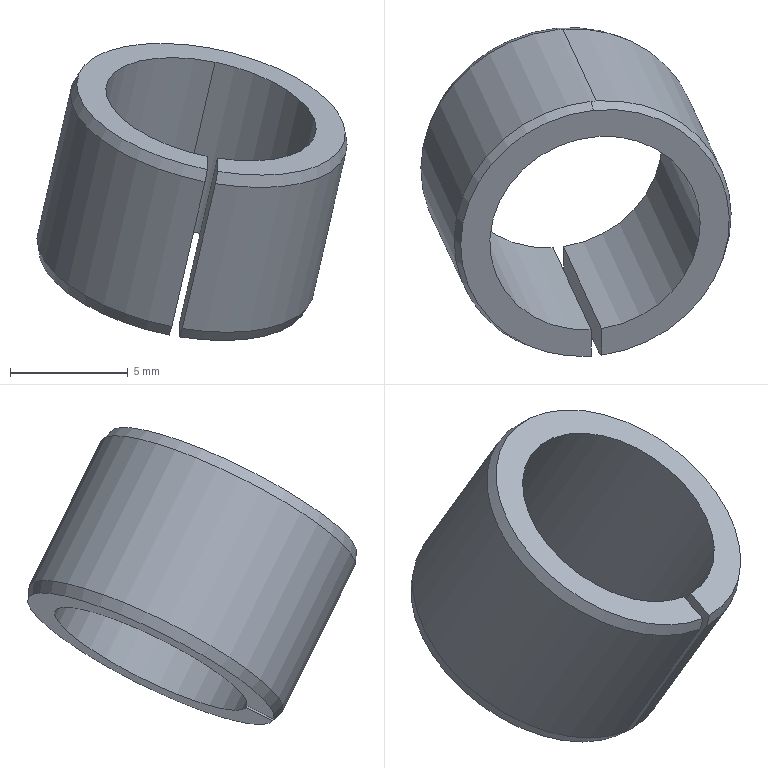Part | SolidWorks | features BaseBody 1 | 1 solid | 12 faces | box 13.154 x 13.951 x 12.601 mm | volume 373.279 mm3 | cone 4 | cylinder 4 | plane 4 | commonest cylinder face diameters 9.11 x2 11.99 x2
STEP:
#1=CARTESIAN_POINT('',(1949.772,-211.955,916.36));
#2=VERTEX_POINT('',#1);
#3=CARTESIAN_POINT('',(1949.419,-201.584,921.597));
#4=VERTEX_POINT('',#3);
#5=CARTESIAN_POINT('',(1949.485,-206.783,918.997));
#6=DIRECTION('',(0.2015,-0.436,0.8771));
#7=DIRECTION('',(0.9794,0.1001,-0.1752));
#8=AXIS2_PLACEMENT_3D('',#5,#6,#7);
#9=CIRCLE('',#8,5.813);
#10=EDGE_CURVE('',#2,#4,#9,.T.);
#11=ORIENTED_EDGE('',*,*,#10,.T.);
#12=CARTESIAN_POINT('',(1949.518,-201.639,922.117));
#13=VERTEX_POINT('',#12);
#14=CARTESIAN_POINT('',(1946.268,-199.819,904.989));
#15=DIRECTION('',(0.1854,-0.1038,0.9772));
#16=VECTOR('',#15,1000.);
#17=LINE('',#14,#16);
#18=EDGE_CURVE('',#4,#13,#17,.T.);
#19=ORIENTED_EDGE('',*,*,#18,.T.);
#20=CARTESIAN_POINT('',(1949.738,-201.62,922.076));
#21=VERTEX_POINT('',#20);
#22=CARTESIAN_POINT('',(1949.586,-207.001,919.436));
#23=DIRECTION('',(0.2015,-0.436,0.8771));
#24=DIRECTION('',(0.9794,0.1001,-0.1752));
#25=AXIS2_PLACEMENT_3D('',#22,#23,#24);
#26=CIRCLE('',#25,5.995);
#27=EDGE_CURVE('',#21,#13,#26,.T.);
#28=ORIENTED_EDGE('',*,*,#27,.F.);
#29=CARTESIAN_POINT('',(1949.875,-212.336,916.717));
#30=VERTEX_POINT('',#29);
#31=CARTESIAN_POINT('',(1949.586,-207.001,919.436));
#32=DIRECTION('',(0.2015,-0.436,0.8771));
#33=DIRECTION('',(0.9794,0.1001,-0.1752));
#34=AXIS2_PLACEMENT_3D('',#31,#32,#33);
#35=CIRCLE('',#34,5.995);
#36=EDGE_CURVE('',#30,#21,#35,.T.);
#37=ORIENTED_EDGE('',*,*,#36,.F.);
#38=CARTESIAN_POINT('',(1949.824,-212.146,916.539));
#39=DIRECTION('',(-0.1932,0.7158,-0.6711));
#40=VECTOR('',#39,1000.);
#41=LINE('',#38,#40);
#42=EDGE_CURVE('',#30,#2,#41,.T.);
#43=ORIENTED_EDGE('',*,*,#42,.T.);
#44=EDGE_LOOP('',(#11,#19,#28,#37,#43));
#45=FACE_OUTER_BOUND('',#44,.T.);
#46=CARTESIAN_POINT('',(2147.735,-635.836,1782.087));
#47=DIRECTION('',(0.2015,-0.436,0.8771));
#48=DIRECTION('',(-0.01144,0.8943,0.4472));
#49=AXIS2_PLACEMENT_3D('',#46,#47,#48);
#50=CONICAL_SURFACE('',#49,363.97,0.3491);
#51=ADVANCED_FACE('',(#45),#50,.T.);
#52=ORIENTED_EDGE('',*,*,#36,.T.);
#53=CARTESIAN_POINT('',(1951.148,-204.672,928.215));
#54=VERTEX_POINT('',#53);
#55=CARTESIAN_POINT('',(1950.443,-203.146,925.145));
#56=DIRECTION('',(0.2015,-0.436,0.8771));
#57=VECTOR('',#56,1000.);
#58=LINE('',#55,#57);
#59=EDGE_CURVE('',#21,#54,#58,.T.);
#60=ORIENTED_EDGE('',*,*,#59,.T.);
#61=CARTESIAN_POINT('',(1951.285,-215.388,922.857));
#62=VERTEX_POINT('',#61);
#63=CARTESIAN_POINT('',(1950.996,-210.053,925.576));
#64=DIRECTION('',(0.2015,-0.436,0.8771));
#65=DIRECTION('',(0.9794,0.1001,-0.1752));
#66=AXIS2_PLACEMENT_3D('',#63,#64,#65);
#67=CIRCLE('',#66,5.995);
#68=EDGE_CURVE('',#62,#54,#67,.T.);
#69=ORIENTED_EDGE('',*,*,#68,.F.);
#70=CARTESIAN_POINT('',(1950.58,-213.862,919.787));
#71=DIRECTION('',(-0.2015,0.436,-0.8771));
#72=VECTOR('',#71,1000.);
#73=LINE('',#70,#72);
#74=EDGE_CURVE('',#62,#30,#73,.T.);
#75=ORIENTED_EDGE('',*,*,#74,.T.);
#76=EDGE_LOOP('',(#52,#60,#69,#75));
#77=FACE_OUTER_BOUND('',#76,.T.);
#78=CARTESIAN_POINT('',(1950.291,-208.527,922.506));
#79=DIRECTION('',(0.2015,-0.436,0.8771));
#80=DIRECTION('',(0.02532,0.8975,0.4403));
#81=AXIS2_PLACEMENT_3D('',#78,#79,#80);
#82=CYLINDRICAL_SURFACE('',#81,5.995);
#83=ADVANCED_FACE('',(#77),#82,.T.);
#84=CARTESIAN_POINT('',(1951.031,-205.072,928.614));
#85=VERTEX_POINT('',#84);
#86=CARTESIAN_POINT('',(1950.943,-215.488,923.456));
#87=VERTEX_POINT('',#86);
#88=CARTESIAN_POINT('',(1951.097,-210.271,926.014));
#89=DIRECTION('',(0.2015,-0.436,0.8771));
#90=DIRECTION('',(0.9794,0.1001,-0.1752));
#91=AXIS2_PLACEMENT_3D('',#88,#89,#90);
#92=CIRCLE('',#91,5.813);
#93=EDGE_CURVE('',#85,#87,#92,.T.);
#94=ORIENTED_EDGE('',*,*,#93,.F.);
#95=CARTESIAN_POINT('',(1950.928,-204.691,928.257));
#96=VERTEX_POINT('',#95);
#97=CARTESIAN_POINT('',(1954.315,-217.234,940.022));
#98=DIRECTION('',(-0.1932,0.7156,-0.6712));
#99=VECTOR('',#98,1000.);
#100=LINE('',#97,#99);
#101=EDGE_CURVE('',#85,#96,#100,.T.);
#102=ORIENTED_EDGE('',*,*,#101,.T.);
#103=CARTESIAN_POINT('',(1950.845,-215.433,922.936));
#104=VERTEX_POINT('',#103);
#105=CARTESIAN_POINT('',(1950.996,-210.053,925.576));
#106=DIRECTION('',(0.2015,-0.436,0.8771));
#107=DIRECTION('',(0.9794,0.1001,-0.1752));
#108=AXIS2_PLACEMENT_3D('',#105,#106,#107);
#109=CIRCLE('',#108,5.995);
#110=EDGE_CURVE('',#96,#104,#109,.T.);
#111=ORIENTED_EDGE('',*,*,#110,.T.);
#112=CARTESIAN_POINT('',(1950.894,-215.461,923.196));
#113=DIRECTION('',(0.1854,-0.1036,0.9772));
#114=VECTOR('',#113,1000.);
#115=LINE('',#112,#114);
#116=EDGE_CURVE('',#104,#87,#115,.T.);
#117=ORIENTED_EDGE('',*,*,#116,.T.);
#118=EDGE_LOOP('',(#94,#102,#111,#117));
#119=FACE_OUTER_BOUND('',#118,.T.);
#120=CARTESIAN_POINT('',(1752.847,218.782,62.925));
#121=DIRECTION('',(-0.2015,0.436,-0.8771));
#122=DIRECTION('',(-0.01144,0.8943,0.4472));
#123=AXIS2_PLACEMENT_3D('',#120,#121,#122);
#124=CONICAL_SURFACE('',#123,363.97,0.3491);
#125=ADVANCED_FACE('',(#119),#124,.T.);
#126=CARTESIAN_POINT('',(1949.317,-210.874,917.002));
#127=VERTEX_POINT('',#126);
#128=CARTESIAN_POINT('',(1949.654,-202.691,920.993));
#129=VERTEX_POINT('',#128);
#130=CARTESIAN_POINT('',(1949.485,-206.783,918.997));
#131=DIRECTION('',(-0.2015,0.436,-0.8771));
#132=DIRECTION('',(0.9794,0.1001,-0.1752));
#133=AXIS2_PLACEMENT_3D('',#130,#131,#132);
#134=CIRCLE('',#133,4.555);
#135=EDGE_CURVE('',#127,#129,#134,.T.);
#136=ORIENTED_EDGE('',*,*,#135,.T.);
#137=CARTESIAN_POINT('',(1951.266,-206.179,928.009));
#138=VERTEX_POINT('',#137);
#139=CARTESIAN_POINT('',(1950.46,-204.435,924.501));
#140=DIRECTION('',(0.2015,-0.436,0.8771));
#141=VECTOR('',#140,1000.);
#142=LINE('',#139,#141);
#143=EDGE_CURVE('',#129,#138,#142,.T.);
#144=ORIENTED_EDGE('',*,*,#143,.T.);
#145=CARTESIAN_POINT('',(1950.929,-214.362,924.019));
#146=VERTEX_POINT('',#145);
#147=CARTESIAN_POINT('',(1951.097,-210.271,926.014));
#148=DIRECTION('',(-0.2015,0.436,-0.8771));
#149=DIRECTION('',(0.9794,0.1001,-0.1752));
#150=AXIS2_PLACEMENT_3D('',#147,#148,#149);
#151=CIRCLE('',#150,4.555);
#152=EDGE_CURVE('',#146,#138,#151,.T.);
#153=ORIENTED_EDGE('',*,*,#152,.F.);
#154=CARTESIAN_POINT('',(1950.123,-212.618,920.511));
#155=DIRECTION('',(-0.2015,0.436,-0.8771));
#156=VECTOR('',#155,1000.);
#157=LINE('',#154,#156);
#158=EDGE_CURVE('',#146,#127,#157,.T.);
#159=ORIENTED_EDGE('',*,*,#158,.T.);
#160=EDGE_LOOP('',(#136,#144,#153,#159));
#161=FACE_OUTER_BOUND('',#160,.T.);
#162=CARTESIAN_POINT('',(1950.291,-208.527,922.506));
#163=DIRECTION('',(0.2015,-0.436,0.8771));
#164=DIRECTION('',(0.03695,0.8982,0.438));
#165=AXIS2_PLACEMENT_3D('',#162,#163,#164);
#166=CYLINDRICAL_SURFACE('',#165,4.555);
#167=ADVANCED_FACE('',(#161),#166,.F.);
#168=ORIENTED_EDGE('',*,*,#143,.F.);
#169=CARTESIAN_POINT('',(1949.758,-210.829,916.923));
#170=VERTEX_POINT('',#169);
#171=CARTESIAN_POINT('',(1949.485,-206.783,918.997));
#172=DIRECTION('',(-0.2015,0.436,-0.8771));
#173=DIRECTION('',(0.9794,0.1001,-0.1752));
#174=AXIS2_PLACEMENT_3D('',#171,#172,#173);
#175=CIRCLE('',#174,4.555);
#176=EDGE_CURVE('',#129,#170,#175,.T.);
#177=ORIENTED_EDGE('',*,*,#176,.T.);
#178=CARTESIAN_POINT('',(1951.37,-214.317,923.94));
#179=VERTEX_POINT('',#178);
#180=CARTESIAN_POINT('',(1950.564,-212.573,920.432));
#181=DIRECTION('',(-0.2015,0.436,-0.8771));
#182=VECTOR('',#181,1000.);
#183=LINE('',#180,#182);
#184=EDGE_CURVE('',#179,#170,#183,.T.);
#185=ORIENTED_EDGE('',*,*,#184,.F.);
#186=CARTESIAN_POINT('',(1951.097,-210.271,926.014));
#187=DIRECTION('',(-0.2015,0.436,-0.8771));
#188=DIRECTION('',(0.9794,0.1001,-0.1752));
#189=AXIS2_PLACEMENT_3D('',#186,#187,#188);
#190=CIRCLE('',#189,4.555);
#191=EDGE_CURVE('',#138,#179,#190,.T.);
#192=ORIENTED_EDGE('',*,*,#191,.F.);
#193=EDGE_LOOP('',(#168,#177,#185,#192));
#194=FACE_OUTER_BOUND('',#193,.T.);
#195=CARTESIAN_POINT('',(1950.291,-208.527,922.506));
#196=DIRECTION('',(0.2015,-0.436,0.8771));
#197=DIRECTION('',(0.03695,0.8982,0.438));
#198=AXIS2_PLACEMENT_3D('',#195,#196,#197);
#199=CYLINDRICAL_SURFACE('',#198,4.555);
#200=ADVANCED_FACE('',(#194),#199,.F.);
#201=CARTESIAN_POINT('',(1951.384,-215.443,923.377));
#202=VERTEX_POINT('',#201);
#203=CARTESIAN_POINT('',(1951.377,-214.88,923.659));
#204=DIRECTION('',(0.01144,-0.8943,-0.4472));
#205=VECTOR('',#204,1000.);
#206=LINE('',#203,#205);
#207=EDGE_CURVE('',#179,#202,#206,.T.);
#208=ORIENTED_EDGE('',*,*,#207,.T.);
#209=CARTESIAN_POINT('',(1951.097,-210.271,926.014));
#210=DIRECTION('',(0.2015,-0.436,0.8771));
#211=DIRECTION('',(0.9794,0.1001,-0.1752));
#212=AXIS2_PLACEMENT_3D('',#209,#210,#211);
#213=CIRCLE('',#212,5.813);
#214=EDGE_CURVE('',#202,#85,#213,.T.);
#215=ORIENTED_EDGE('',*,*,#214,.T.);
#216=ORIENTED_EDGE('',*,*,#93,.T.);
#217=CARTESIAN_POINT('',(1950.936,-214.925,923.737));
#218=DIRECTION('',(-0.01144,0.8943,0.4472));
#219=VECTOR('',#218,1000.);
#220=LINE('',#217,#219);
#221=EDGE_CURVE('',#87,#146,#220,.T.);
#222=ORIENTED_EDGE('',*,*,#221,.T.);
#223=ORIENTED_EDGE('',*,*,#152,.T.);
#224=ORIENTED_EDGE('',*,*,#191,.T.);
#225=EDGE_LOOP('',(#208,#215,#216,#222,#223,#224));
#226=FACE_OUTER_BOUND('',#225,.T.);
#227=CARTESIAN_POINT('',(1951.097,-210.271,926.014));
#228=DIRECTION('',(0.2015,-0.436,0.8771));
#229=DIRECTION('',(-0.9794,-0.1001,0.1752));
#230=AXIS2_PLACEMENT_3D('',#227,#228,#229);
#231=PLANE('',#230);
#232=ADVANCED_FACE('',(#226),#231,.T.);
#233=ORIENTED_EDGE('',*,*,#101,.F.);
#234=ORIENTED_EDGE('',*,*,#214,.F.);
#235=CARTESIAN_POINT('',(1951.335,-215.416,923.117));
#236=DIRECTION('',(-0.1854,0.1036,-0.9772));
#237=VECTOR('',#236,1000.);
#238=LINE('',#235,#237);
#239=EDGE_CURVE('',#202,#62,#238,.T.);
#240=ORIENTED_EDGE('',*,*,#239,.T.);
#241=ORIENTED_EDGE('',*,*,#68,.T.);
#242=CARTESIAN_POINT('',(1950.996,-210.053,925.576));
#243=DIRECTION('',(0.2015,-0.436,0.8771));
#244=DIRECTION('',(0.9794,0.1001,-0.1752));
#245=AXIS2_PLACEMENT_3D('',#242,#243,#244);
#246=CIRCLE('',#245,5.995);
#247=EDGE_CURVE('',#54,#96,#246,.T.);
#248=ORIENTED_EDGE('',*,*,#247,.T.);
#249=EDGE_LOOP('',(#233,#234,#240,#241,#248));
#250=FACE_OUTER_BOUND('',#249,.T.);
#251=CARTESIAN_POINT('',(1752.847,218.782,62.925));
#252=DIRECTION('',(-0.2015,0.436,-0.8771));
#253=DIRECTION('',(-0.01144,0.8943,0.4472));
#254=AXIS2_PLACEMENT_3D('',#251,#252,#253);
#255=CONICAL_SURFACE('',#254,363.97,0.3491);
#256=ADVANCED_FACE('',(#250),#255,.T.);
#257=ORIENTED_EDGE('',*,*,#10,.F.);
#258=CARTESIAN_POINT('',(1949.765,-211.392,916.642));
#259=DIRECTION('',(0.01144,-0.8943,-0.4472));
#260=VECTOR('',#259,1000.);
#261=LINE('',#258,#260);
#262=EDGE_CURVE('',#170,#2,#261,.T.);
#263=ORIENTED_EDGE('',*,*,#262,.F.);
#264=ORIENTED_EDGE('',*,*,#176,.F.);
#265=ORIENTED_EDGE('',*,*,#135,.F.);
#266=CARTESIAN_POINT('',(1949.332,-212.,916.439));
#267=VERTEX_POINT('',#266);
#268=CARTESIAN_POINT('',(1949.324,-211.437,916.721));
#269=DIRECTION('',(-0.01144,0.8943,0.4472));
#270=VECTOR('',#269,1000.);
#271=LINE('',#268,#270);
#272=EDGE_CURVE('',#267,#127,#271,.T.);
#273=ORIENTED_EDGE('',*,*,#272,.F.);
#274=CARTESIAN_POINT('',(1949.485,-206.783,918.997));
#275=DIRECTION('',(0.2015,-0.436,0.8771));
#276=DIRECTION('',(0.9794,0.1001,-0.1752));
#277=AXIS2_PLACEMENT_3D('',#274,#275,#276);
#278=CIRCLE('',#277,5.813);
#279=EDGE_CURVE('',#4,#267,#278,.T.);
#280=ORIENTED_EDGE('',*,*,#279,.F.);
#281=EDGE_LOOP('',(#257,#263,#264,#265,#273,#280));
#282=FACE_OUTER_BOUND('',#281,.T.);
#283=CARTESIAN_POINT('',(1949.485,-206.783,918.997));
#284=DIRECTION('',(0.2015,-0.436,0.8771));
#285=DIRECTION('',(-0.9794,-0.1001,0.1752));
#286=AXIS2_PLACEMENT_3D('',#283,#284,#285);
#287=PLANE('',#286);
#288=ADVANCED_FACE('',(#282),#287,.F.);
#289=ORIENTED_EDGE('',*,*,#59,.F.);
#290=ORIENTED_EDGE('',*,*,#27,.T.);
#291=CARTESIAN_POINT('',(1949.434,-212.381,916.796));
#292=VERTEX_POINT('',#291);
#293=CARTESIAN_POINT('',(1949.586,-207.001,919.436));
#294=DIRECTION('',(0.2015,-0.436,0.8771));
#295=DIRECTION('',(0.9794,0.1001,-0.1752));
#296=AXIS2_PLACEMENT_3D('',#293,#294,#295);
#297=CIRCLE('',#296,5.995);
#298=EDGE_CURVE('',#13,#292,#297,.T.);
#299=ORIENTED_EDGE('',*,*,#298,.T.);
#300=CARTESIAN_POINT('',(1950.14,-213.907,919.866));
#301=DIRECTION('',(-0.2015,0.436,-0.8771));
#302=VECTOR('',#301,1000.);
#303=LINE('',#300,#302);
#304=EDGE_CURVE('',#104,#292,#303,.T.);
#305=ORIENTED_EDGE('',*,*,#304,.F.);
#306=ORIENTED_EDGE('',*,*,#110,.F.);
#307=ORIENTED_EDGE('',*,*,#247,.F.);
#308=EDGE_LOOP('',(#289,#290,#299,#305,#306,#307));
#309=FACE_OUTER_BOUND('',#308,.T.);
#310=CARTESIAN_POINT('',(1950.291,-208.527,922.506));
#311=DIRECTION('',(0.2015,-0.436,0.8771));
#312=DIRECTION('',(0.02532,0.8975,0.4403));
#313=AXIS2_PLACEMENT_3D('',#310,#311,#312);
#314=CYLINDRICAL_SURFACE('',#313,5.995);
#315=ADVANCED_FACE('',(#309),#314,.T.);
#316=ORIENTED_EDGE('',*,*,#262,.T.);
#317=ORIENTED_EDGE('',*,*,#42,.F.);
#318=ORIENTED_EDGE('',*,*,#74,.F.);
#319=ORIENTED_EDGE('',*,*,#239,.F.);
#320=ORIENTED_EDGE('',*,*,#207,.F.);
#321=ORIENTED_EDGE('',*,*,#184,.T.);
#322=EDGE_LOOP('',(#316,#317,#318,#319,#320,#321));
#323=FACE_OUTER_BOUND('',#322,.T.);
#324=CARTESIAN_POINT('',(1950.58,-213.862,919.787));
#325=DIRECTION('',(-0.9794,-0.1001,0.1752));
#326=DIRECTION('',(0.01144,-0.8943,-0.4472));
#327=AXIS2_PLACEMENT_3D('',#324,#325,#326);
#328=PLANE('',#327);
#329=ADVANCED_FACE('',(#323),#328,.T.);
#330=CARTESIAN_POINT('',(1949.383,-212.191,916.617));
#331=DIRECTION('',(0.1932,-0.7158,0.6711));
#332=VECTOR('',#331,1000.);
#333=LINE('',#330,#332);
#334=EDGE_CURVE('',#267,#292,#333,.T.);
#335=ORIENTED_EDGE('',*,*,#334,.F.);
#336=ORIENTED_EDGE('',*,*,#272,.T.);
#337=ORIENTED_EDGE('',*,*,#158,.F.);
#338=ORIENTED_EDGE('',*,*,#221,.F.);
#339=ORIENTED_EDGE('',*,*,#116,.F.);
#340=ORIENTED_EDGE('',*,*,#304,.T.);
#341=EDGE_LOOP('',(#335,#336,#337,#338,#339,#340));
#342=FACE_OUTER_BOUND('',#341,.T.);
#343=CARTESIAN_POINT('',(1950.14,-213.907,919.866));
#344=DIRECTION('',(-0.9794,-0.1001,0.1752));
#345=DIRECTION('',(0.01144,-0.8943,-0.4472));
#346=AXIS2_PLACEMENT_3D('',#343,#344,#345);
#347=PLANE('',#346);
#348=ADVANCED_FACE('',(#342),#347,.F.);
#349=ORIENTED_EDGE('',*,*,#18,.F.);
#350=ORIENTED_EDGE('',*,*,#279,.T.);
#351=ORIENTED_EDGE('',*,*,#334,.T.);
#352=ORIENTED_EDGE('',*,*,#298,.F.);
#353=EDGE_LOOP('',(#349,#350,#351,#352));
#354=FACE_OUTER_BOUND('',#353,.T.);
#355=CARTESIAN_POINT('',(2147.735,-635.836,1782.087));
#356=DIRECTION('',(0.2015,-0.436,0.8771));
#357=DIRECTION('',(-0.01144,0.8943,0.4472));
#358=AXIS2_PLACEMENT_3D('',#355,#356,#357);
#359=CONICAL_SURFACE('',#358,363.97,0.3491);
#360=ADVANCED_FACE('',(#354),#359,.T.);
#361=CLOSED_SHELL('',(#51,#83,#125,#167,#200,#232,#256,#288,#315,#329,#348,#360));
#362=MANIFOLD_SOLID_BREP('',#361);
#363=CARTESIAN_POINT('',(0.,0.,0.));
#364=DIRECTION('',(0.,0.,1.));
#365=DIRECTION('',(1.,0.,0.));
#366=AXIS2_PLACEMENT_3D('',#363,#364,#365);
#367=(LENGTH_UNIT()NAMED_UNIT(*)SI_UNIT(.MILLI.,.METRE.));
#368=UNCERTAINTY_MEASURE_WITH_UNIT(LENGTH_MEASURE(0.00001),#367,'','');
#369=(NAMED_UNIT(*)PLANE_ANGLE_UNIT()SI_UNIT($,.RADIAN.));
#370=(NAMED_UNIT(*)SI_UNIT($,.STERADIAN.)SOLID_ANGLE_UNIT());
#371=(GEOMETRIC_REPRESENTATION_CONTEXT(3)GLOBAL_UNCERTAINTY_ASSIGNED_CONTEXT((#368))GLOBAL_UNIT_ASSIGNED_CONTEXT((#367,#369,#370))REPRESENTATION_CONTEXT('',''));
#372=ADVANCED_BREP_SHAPE_REPRESENTATION('',(#362,#366),#371);